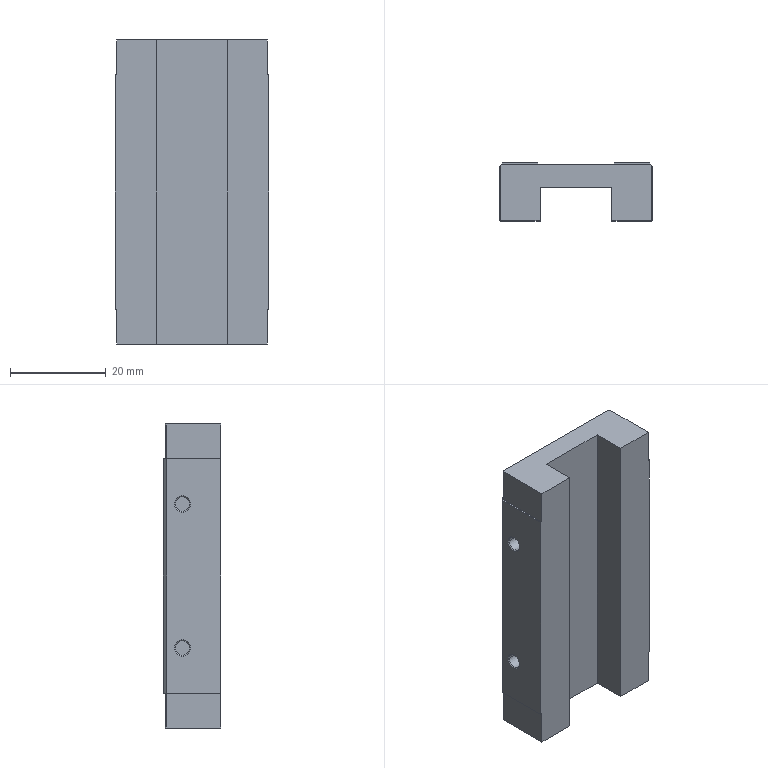Part | 1 solid | 87 faces | box 32 x 12 x 63.4 mm | volume 16775 mm3 | plane 42 | cylinder 25 | cone 20 | commonest cylinder face diameters 4 x12 3 x9 2 x4